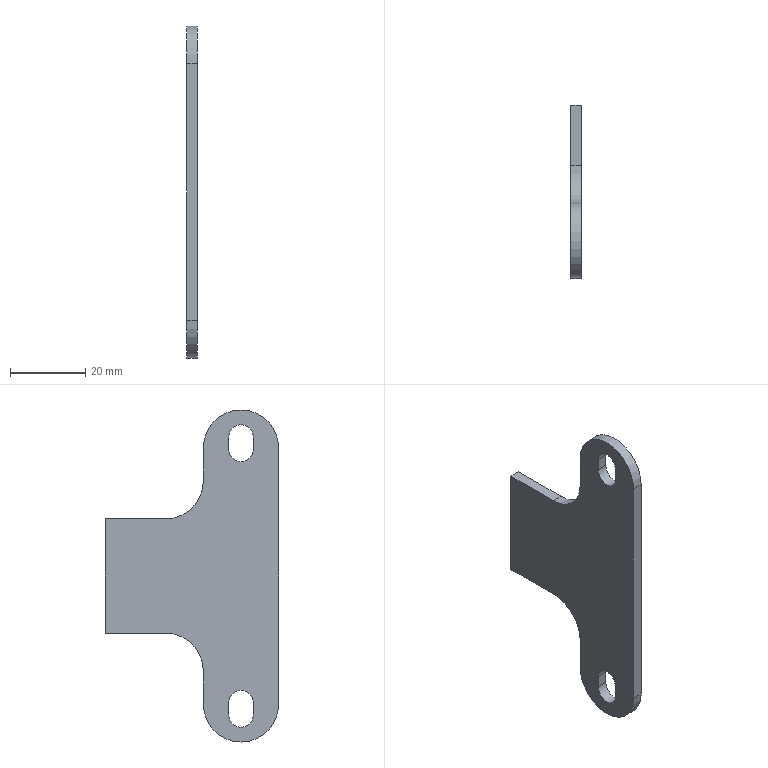Part | STEP file | PRT0001_68_23 | 1 solid | 20 faces | box 2.865 x 46.012 x 88.1 mm | volume 6874 mm3 | plane 12 | cylinder 8 | commonest cylinder face diameters 6.5 x4 20 x4